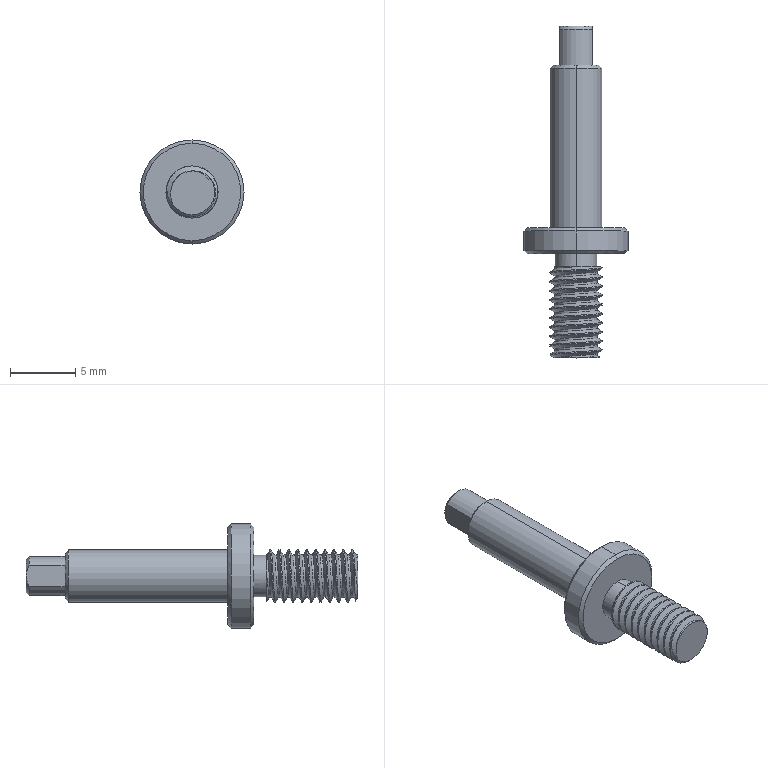Part | NX | features BREP 1 | 1 solid | 50 faces | box 8 x 25.5 x 8 mm | volume 353.749 mm3 | cylinder 30 | cone 10 | plane 8 | spline 2 | commonest cylinder face diameters 4 x22 3 x3 3.2 x2 8 x2 3.242 x1